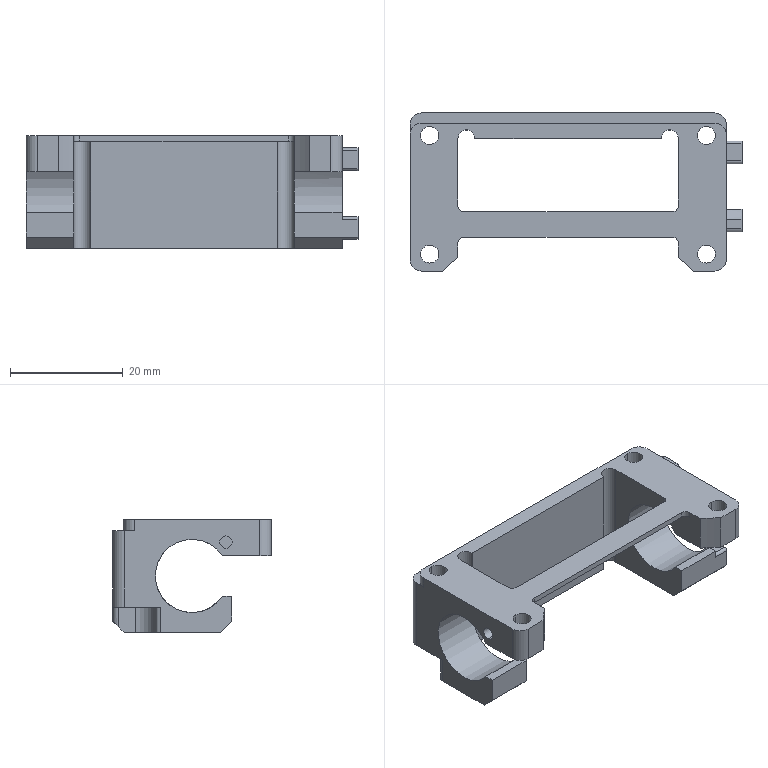NC program | Mastercam | posted with a generic post | part box 58.8 x 28 x 20 mm
Lines 58 to 1155 of 29451:
(10 FEM |TOOL - 10|DIA. OFF. - 10|LEN. - 10|TOOL DIA. - 10.)
N182 T10 M6
N184 G0 G54 G90 X44.9 Y11.6 C0. B0. S6500 M3
N186 G43 H10 Z25.
N188 Z5.
N190 G1 Z0. F600.
N192 X34.9 F4000.
N194 X28.421
N196 X27.5
N198 G3 X27.503 Y11.8 I-6.677 J.2
N200 X27.331 Y13.306 I-6.68
N202 X22.397 Y17.14 I-4.94 J-1.266
N204 G1 X-19.603
N206 G3 X-24.686 Y12.372 I.004 J-5.098
N208 X-24.702 Y11.824 I9.387 J-.548
N210 X-24.7 Y11.6 I9.403
N212 X-25.137 Y11.607 I-.437 J-14.093
N214 X-26.331 Y11.556 J-14.1
N216 X-31.497 Y7.059 I.769 J-6.099
N218 X-31.7 Y5.553 I6.076 J-1.583
N220 G1 Y-4.947
N222 Y-4.999
N224 G3 X-26.909 Y-10.131 I5.144
N226 G1 X-26.591 Y-10.14
N228 X-18.113
N230 G3 X-13.146 Y-6.056 I-.016 J5.083
N232 X-13.035 Y-4.999 I-4.996 J1.057
N234 G1 Y-4.967
N236 Y4.401
N238 X15.835
N240 Y-4.947
N242 Y-4.999
N244 G3 X20.626 Y-10.131 I5.144
N246 G1 X20.944 Y-10.14
N248 X29.422
N250 G3 X34.389 Y-6.056 I-.016 J5.083
N252 X34.5 Y-4.999 I-4.993 J1.057
N254 G1 Y-4.976
N256 Y5.5
N258 G3 X30.664 Y11.164 I-6.149 J-.033
N260 X28.421 Y11.6 I-2.297 J-5.835
N262 G2 X30.664 Y11.164 I-.054 J-6.271
N264 X34.5 Y5.5 I-2.313 J-5.697
N266 G1 Y-4.976
N268 Y-4.999
N270 G2 X34.389 Y-6.056 I-5.104
N272 X29.422 Y-10.14 I-4.983 J.999
N274 G1 X20.944
N276 X20.626 Y-10.131
N278 G2 X15.835 Y-4.999 I.353 J5.132
N280 G1 Y-4.947
N282 Y2.121
N284 X1.735 Y-8.5
N286 X.501 Y-9.
N288 X2.308
N290 X9.335 Y-2.
N292 X-6.535
N294 X-6.035 Y-3.5
N296 Y-5.
N298 X-6.048 Y-5.5
N300 X-6.087 Y-6.
N302 X-6.203 Y-7.
N304 X-6.296 Y-7.5
N306 X-6.414 Y-8.
N308 X-6.56 Y-8.5
N310 X-6.895 Y-9.5
N312 X-7.104 Y-10.
N314 X-7.347 Y-10.5
N316 X-7.628 Y-11.
N318 X-8.242 Y-12.
N320 X-9.644 Y-13.
N322 X-13.997 Y-14.5
N324 X-28.109 Y-15.
N326 X27.9
N328 X16.824 Y-14.5
N330 X12.468 Y-13.
N332 X11.058 Y-12.
N334 X10.733 Y-11.5
N336 X10.158 Y-10.5
N338 X9.913 Y-10.
N340 X9.702 Y-9.5
N342 X9.523 Y-9.
N344 X9.215 Y-8.
N346 X9.095 Y-7.5
N348 X9.003 Y-7.
N350 X8.938 Y-6.5
N352 X8.848 Y-5.5
N354 X8.835 Y-5.
N356 Y-4.
N358 X9.335 Y-2.
N360 X16.101 Y-6.631
N362 G3 X20.626 Y-10.131 I4.878 J1.632
N364 G1 X20.944 Y-10.14
N366 X21.227
N368 X34.9 Y-19.5
N370 Y19.5
N372 X-34.9
N374 Y-19.5
N376 X34.9
N378 G0 Z5.
N380 Z25.
N382 X44.9 Y11.6
N384 Z4.414
N386 G1 Z-.586 F600.
N388 X34.9 F4000.
N390 X28.426
N392 X27.5
N394 G3 X27.509 Y12.093 I-12.959 J.493
N396 X27.46 Y13.223 I-12.968
N398 X23.346 Y17.637 I-5.119 J-.647
N400 X22.4 Y17.726 I-.946 J-4.973
N402 G1 X22.397
N404 X-19.603
N406 G3 X-24.686 Y12.957 I.004 J-5.098
N408 X-24.708 Y12.119 I16.278 J-.838
N410 X-24.7 Y11.6 I16.3
N412 X-25.137 Y11.607 I-.437 J-13.987
N414 X-26.336 Y11.555 J-13.994
N416 X-31.57 Y6.748 I.77 J-6.091
N418 X-31.7 Y5.553 I7.039 J-1.369
N420 G1 Y-5.533
N422 Y-5.585
N424 G3 X-26.909 Y-10.717 I5.144
N426 G1 X-26.591 Y-10.726
N428 X-18.126
N430 G3 X-13.053 Y-6.01 I-.01 J5.098
N432 X-13.035 Y-5.586 I-5.082 J.424
N434 G1 Y4.401
N436 X15.835
N438 Y-5.533
N440 Y-5.585
N442 G3 X20.626 Y-10.717 I5.144
N444 G1 X20.944 Y-10.726
N446 X29.409
N448 G3 X34.482 Y-6.01 I-.01 J5.098
N450 X34.5 Y-5.586 I-5.082 J.424
N452 G1 Y5.504
N454 G3 X30.364 Y11.274 I-6.14 J-.034
N456 X28.426 Y11.6 I-2.012 J-6.031
N458 G1 X27.5
N460 X28.426
N462 G2 X30.364 Y11.274 I-.074 J-6.357
N464 X34.5 Y5.504 I-2.004 J-5.804
N466 G1 Y-5.586
N468 G2 X34.482 Y-6.01 I-5.1
N470 X29.409 Y-10.726 I-5.083 J.382
N472 G1 X20.944
N474 X20.626 Y-10.717
N476 G2 X15.835 Y-5.585 I.353 J5.132
N478 G1 Y-5.533
N480 Y4.401
N482 X12.048
N484 X-13.372 Y-7.443
N486 G2 X-18.126 Y-10.726 I-4.764 J1.815
N488 G1 X-20.418
N490 X-29.591 Y-15.
N492 X1.663 Y-8.5
N494 X.805
N496 X2.001
N498 X9.335 Y-2.
N500 X-6.535
N502 X-6.035 Y-3.5
N504 Y-5.5
N506 X-6.044 Y-6.
N508 X-6.078 Y-6.5
N510 X-6.187 Y-7.5
N512 X-6.273 Y-8.
N514 X-6.387 Y-8.5
N516 X-6.529 Y-9.
N518 X-6.859 Y-10.
N520 X-7.063 Y-10.5
N522 X-7.301 Y-11.
N524 X-7.575 Y-11.5
N526 X-8.986 Y-13.
N528 X-13.615 Y-14.5
N530 X16.441
N532 X11.807 Y-13.
N534 X10.682 Y-12.
N536 X10.114 Y-11.
N538 X9.874 Y-10.5
N540 X9.669 Y-10.
N542 X9.495 Y-9.5
N544 X9.193 Y-8.5
N546 X9.078 Y-8.
N548 X8.99 Y-7.5
N550 X8.929 Y-7.
N552 X8.844 Y-6.
N554 X8.835 Y-5.5
N556 Y-3.5
N558 X9.335 Y-2.
N560 X15.918 Y-6.506
N562 G3 X20.626 Y-10.717 I5.061 J.921
N564 G1 X20.944 Y-10.726
N566 X22.083
N568 X34.9 Y-19.5
N570 Y19.5
N572 X-34.9
N574 Y-19.5
N576 X34.9
N578 G0 Z4.414
N580 Z25.
N582 X27.236 Y29.5
N584 Z3.829
N586 G1 Z-1.171 F600.
N588 Y19.5 F4000.
N590 Y14.741
N592 G3 X25.868 Y16.918 I-5.03 J-1.642
N594 X22.365 Y18.311 I-3.508 J-3.723
N596 G1 X3.073 Y18.312
N598 X1.823 Y18.313
N600 X-4.083 Y18.312
N602 G3 X-5.36 Y18.313 I-1.277 J-732.939
N604 X-6.588 Y18.312 J-732.94
N606 X-7.288 Y18.313 I-.7 J-235.219
N608 X-8.017 Y18.312 J-235.22
N610 X-8.697 Y18.313 I-.68 J-317.868
N612 X-9.377 Y18.312 J-317.869
N614 G1 X-19.388
N616 X-19.408
N618 X-19.438
N620 X-19.457 Y18.313
N622 X-19.476 Y18.312
N624 X-19.499 Y18.313
N626 G3 X-21.136 Y18.062 I.07 J-5.92
N628 X-24.686 Y13.372 I1.604 J-4.903
N630 G1 X-24.7 Y13.053
N632 Y11.6
N634 G3 X-25.137 Y11.607 I-.437 J-14.066
N636 X-26.331 Y11.556 J-14.073
N638 X-31.497 Y7.059 I.769 J-6.099
N640 X-31.7 Y5.553 I6.075 J-1.583
N642 G1 Y-6.119
N644 Y-6.17
N646 G3 X-26.909 Y-11.302 I5.144
N648 G1 X-26.591 Y-11.312
N650 X-18.126
N652 G3 X-13.053 Y-6.596 I-.01 J5.098
N654 X-13.035 Y-6.171 I-5.082 J.425
N656 G1 Y4.401
N658 X15.835
N660 Y-6.119
N662 Y-6.17
N664 G3 X20.626 Y-11.302 I5.144
N666 G1 X20.944 Y-11.312
N668 X29.409
N670 G3 X34.482 Y-6.596 I-.01 J5.098
N672 X34.5 Y-6.171 I-5.082 J.425
N674 G1 Y5.509
N676 G3 X29.934 Y11.404 I-6.137 J-.037
N678 X28.426 Y11.6 I-1.564 J-6.137
N680 G1 X27.5
N682 G3 X27.509 Y12.3 I-27.475 J.7
N684 X27.49 Y13.319 I-27.484
N686 X27.236 Y14.741 I-5.705 J-.284
N688 G2 X27.49 Y13.319 I-5.451 J-1.706
N690 X27.509 Y12.3 I-27.465 J-1.019
N692 X27.5 Y11.6 I-27.484
N694 G1 X28.426
N696 G2 X29.934 Y11.404 I-.056 J-6.333
N698 X34.5 Y5.509 I-1.571 J-5.932
N700 G1 Y-6.171
N702 G2 X34.482 Y-6.596 I-5.1
N704 X29.409 Y-11.312 I-5.083 J.382
N706 G1 X20.944
N708 X20.626 Y-11.302
N710 G2 X15.835 Y-6.17 I.353 J5.132
N712 G1 Y-6.119
N714 Y4.4
N716 X1.614 Y-8.5
N718 X.934
N720 X1.87
N722 X9.335 Y-2.
N724 X-6.535
N726 X-6.035 Y-3.5
N728 Y-6.
N730 X-6.041 Y-6.5
N732 X-6.071 Y-7.
N734 X-6.175 Y-8.
N736 X-6.257 Y-8.5
N738 X-6.365 Y-9.
N740 X-6.502 Y-9.5
N742 X-6.827 Y-10.5
N744 X-7.025 Y-11.
N746 X-7.257 Y-11.5
N748 X-8.029 Y-12.5
N750 X-11.823 Y-14.5
N752 X14.65
N754 X10.847 Y-12.5
N756 X10.07 Y-11.5
N758 X9.837 Y-11.
N760 X9.637 Y-10.5
N762 X9.468 Y-10.
N764 X9.171 Y-9.
N766 X9.061 Y-8.5
N768 X8.978 Y-8.
N770 X8.921 Y-7.5
N772 X8.841 Y-6.5
N774 X8.835 Y-6.
N776 Y-3.5
N778 X9.335 Y-2.
N780 X15.843 Y-6.455
N782 G3 X20.626 Y-11.302 I5.136 J.285
N784 G1 X20.944 Y-11.312
N786 X22.938
N788 X34.9 Y-19.5
N790 Y19.5
N792 X-34.9
N794 Y-19.5
N796 X34.9
N798 G0 Z3.829
N800 Z25.
N802 X25.369 Y29.5
N804 Z3.243
N806 G1 Z-1.757 F600.
N808 Y19.5 F4000.
N810 Y17.627
N812 G3 X21.945 Y18.898 I-3.424 J-3.975
N814 G1 X21.94
N816 G3 X20.816 Y18.9 I-1.124 J-452.637
N818 X19.19 Y18.898 J-452.638
N820 X17.39 Y18.903 I-1.8 J-322.689
N822 X15.589 Y18.898 J-322.694
N824 G1 X-18.884
N826 G3 X-19.084 Y18.902 I-.2 J-5.411
N828 X-22.47 Y17.712 J-5.415
N830 X-24.7 Y13.053 I3.808 J-4.686
N832 G1 Y11.6
N834 G3 X-25.138 Y11.607 I-.438 J-14.051
N836 X-26.331 Y11.556 J-14.058
N838 X-31.497 Y7.059 I.769 J-6.099
N840 X-31.7 Y5.553 I6.075 J-1.583
N842 G1 Y1.439
N844 G3 X-33.303 Y.168 I2.049 J-4.231
N846 X-34.5 Y-3.094 I3.939 J-3.295
N848 G1 Y-6.704
N850 Y-6.756
N852 G3 X-29.709 Y-11.888 I5.144
N854 G1 X-29.391 Y-11.898
N856 X-18.126
N858 G3 X-13.053 Y-7.181 I-.01 J5.098
N860 X-13.035 Y-6.757 I-5.082 J.424
N862 G1 Y4.401
N864 X15.835
N866 Y-6.704
N868 Y-6.756
N870 G3 X20.626 Y-11.888 I5.144
N872 G1 X20.944 Y-11.898
N874 X29.409
N876 G3 X34.482 Y-7.181 I-.01 J5.098
N878 X34.5 Y-6.757 I-5.082 J.424
N880 G1 Y5.513
N882 G3 X29.184 Y11.549 I-6.13 J-.039
N884 X28.426 Y11.6 I-.829 J-6.718
N886 G1 X27.5
N888 G3 X27.509 Y12.299 I-27.561 J.699
N890 X27.49 Y13.319 I-27.57
N892 X25.369 Y17.627 I-6.057 J-.305
N894 G2 X27.49 Y13.319 I-3.936 J-4.613
N896 X27.509 Y12.299 I-27.551 J-1.02
N898 X27.5 Y11.6 I-27.57
N900 G1 X28.426
N902 G2 X29.184 Y11.549 I-.071 J-6.769
N904 X34.5 Y5.513 I-.814 J-6.075
N906 G1 Y-6.757
N908 G2 X34.482 Y-7.181 I-5.1
N910 X29.409 Y-11.898 I-5.083 J.381
N912 G1 X20.944
N914 X20.626 Y-11.888
N916 G2 X15.835 Y-6.756 I.353 J5.132
N918 G1 Y-6.704
N920 Y4.401
N922 X13.005
N924 X1.412 Y-8.
N926 X1.392
N928 X1.249 Y-8.5
N930 X1.542
N932 X1.412 Y-8.
N934 X9.335 Y-2.
N936 X-6.535
N938 X-6.035 Y-3.5
N940 Y-6.5
N942 X-6.038 Y-7.
N944 X-6.064 Y-7.5
N946 X-6.114 Y-8.
N948 X-6.241 Y-9.
N950 X-6.344 Y-9.5
N952 X-6.477 Y-10.
N954 X-6.796 Y-11.
N956 X-6.989 Y-11.5
N958 X-7.215 Y-12.
N960 X-7.477 Y-12.5
N962 X-10.857 Y-14.
N964 X13.683
N966 X10.582 Y-13.
N968 X10.028 Y-12.
N970 X9.8 Y-11.5
N972 X9.606 Y-11.
N974 X9.442 Y-10.5
N976 X9.15 Y-9.5
N978 X9.044 Y-9.
N980 X8.966 Y-8.5
N982 X8.914 Y-8.
N984 X8.838 Y-7.
N986 X8.835 Y-6.5
N988 Y-3.5
N990 X9.335 Y-2.
N992 X15.835 Y-6.449
N994 Y-6.704
N996 Y-6.756
N998 G3 X20.626 Y-11.888 I5.144
N1000 G1 X20.944 Y-11.898
N1002 X23.794
N1004 X34.9 Y-19.5
N1006 Y19.5
N1008 X-34.9
N1010 Y-19.5
N1012 X34.9
N1014 G0 Z3.243
N1016 Z25.
N1018 X23.661 Y29.5
N1020 Z2.657
N1022 G1 Z-2.343 F600.
N1024 Y19.5 F4000.
N1026 Y18.665
N1028 G3 X21.426 Y19.1 I-2.298 J-5.855
N1030 G1 X-18.576
N1032 G3 X-24.647 Y13.801 I.002 J-6.129
N1034 X-24.7 Y13.053 I6.469 J-.833
N1036 G1 Y11.6
N1038 G3 X-25.138 Y11.607 I-.438 J-14.035
N1040 X-26.331 Y11.556 J-14.042
N1042 X-31.497 Y7.059 I.769 J-6.099
N1044 X-31.7 Y5.553 I6.075 J-1.583
N1046 G1 Y1.549
N1048 G3 X-33.304 Y.281 I2.051 J-4.243
N1050 X-34.5 Y-2.956 I3.901 J-3.28
N1052 G1 Y-6.947
N1054 Y-6.999
N1056 G3 X-29.479 Y-12.099 I5.101
N1058 G1 X-18.212
N1060 G3 X-18.134 Y-12.1 I.078 J5.098
N1062 X-13.035 Y-7.001 J5.099
N1064 G1 Y-7.
N1066 Y4.401
N1068 X15.835
N1070 Y-6.947
N1072 Y-6.999
N1074 G3 X20.856 Y-12.099 I5.101
N1076 G1 X29.323
N1078 G3 X29.401 Y-12.1 I.078 J5.098
N1080 X34.5 Y-7.001 J5.099
N1082 G1 Y-7.
N1084 Y5.5
N1086 G3 X30.664 Y11.164 I-6.148 J-.033
N1088 X28.426 Y11.6 I-2.297 J-5.835
N1090 G1 X27.5
N1092 G3 X27.509 Y12.299 I-27.648 J.699
N1094 X27.49 Y13.319 I-27.657
N1096 X23.661 Y18.665 I-6.075 J-.306
N1098 G2 X27.49 Y13.319 I-2.246 J-5.652
N1100 X27.509 Y12.299 I-27.638 J-1.02
N1102 X27.5 Y11.6 I-27.657
N1104 G1 X28.426
N1106 G2 X30.664 Y11.164 I-.059 J-6.271
N1108 X34.5 Y5.5 I-2.312 J-5.697
N1110 G1 Y-7.
N1112 Y-7.001
N1114 G2 X29.401 Y-12.1 I-5.099
N1116 X29.323 Y-12.099 J5.099
N1118 G1 X20.856
N1120 G2 X15.835 Y-6.999 I.08 J5.1
N1122 G1 X15.836 Y-6.947
N1124 X15.835 Y4.401
N1126 X11.751
N1128 X1.397 Y-8.
N1130 X1.28 Y-8.5
N1132 X1.513
N1134 X1.397 Y-8.
N1136 X9.335 Y-2.
N1138 X-6.535
N1140 X-6.035 Y-3.5
N1142 Y-7.
N1144 X-6.048 Y-7.5
N1146 X-6.087 Y-8.
N1148 X-6.203 Y-9.
N1150 X-6.296 Y-9.5
N1152 X-6.416 Y-10.
N1154 X-6.566 Y-10.5
N1156 X-6.904 Y-11.5
N1158 X-7.116 Y-12.
N1160 X-7.363 Y-12.5
N1162 X-10.536 Y-14.
N1164 X13.338
N1166 X10.164 Y-12.5
N1168 X9.917 Y-12.
N1170 X9.705 Y-11.5
N1172 X9.525 Y-11.
N1174 X9.217 Y-10.
N1176 X9.096 Y-9.5
N1178 X9.004 Y-9.
N1180 X8.938 Y-8.5
N1182 X8.848 Y-7.5
N1184 X8.835 Y-7.
N1186 Y-3.5
N1188 X9.335 Y-2.
N1190 X15.835 Y-6.449
N1192 Y-6.947
N1194 Y-6.999
N1196 G3 X20.856 Y-12.099 I5.101
N1198 G1 X24.089
N1200 X34.9 Y-19.5
N1202 Y19.5
N1204 X-34.9
N1206 Y-19.5
N1208 X34.9
N1210 G0 Z2.657
N1212 Z25.
N1214 X23.957 Y29.5
N1216 Z2.071
N1218 G1 Z-2.929 F600.
N1220 Y19.5 F4000.
N1222 Y18.536
N1224 G3 X21.426 Y19.1 I-2.562 J-5.537
N1226 G1 X-18.581
N1228 G3 X-24.7 Y13.053 I.004 J-6.124
N1230 G1 Y11.6
N1232 G3 X-25.137 Y11.607 I-.437 J-14.093
N1234 X-26.331 Y11.556 J-14.1
N1236 X-31.497 Y7.059 I.769 J-6.099
N1238 X-31.7 Y5.553 I6.075 J-1.583
N1240 G1 Y1.549
N1242 G3 X-33.307 Y.278 I2.07 J-4.268
N1244 X-34.5 Y-2.956 I3.898 J-3.275
N1246 G1 Y-6.947
N1248 X-34.469 Y-7.56
N1250 X-34.365 Y-8.165
N1252 X-34.189 Y-8.753
N1254 X-33.943 Y-9.316
N1256 X-33.632 Y-9.845
N1258 X-33.26 Y-10.333
N1260 X-32.831 Y-10.772
N1262 X-32.353 Y-11.157
N1264 X-31.832 Y-11.482
N1266 X-31.276 Y-11.742
N1268 X-30.693 Y-11.934
N1270 X-30.091 Y-12.054
N1272 X-29.479 Y-12.099
N1274 X-18.207
N1276 G3 X-18.131 Y-12.1 I.076 J5.096
N1278 X-13.034 Y-7.003 J5.097
N1280 G1 Y-7.
N1282 X-13.035 Y4.401
N1284 X15.835
N1286 Y-6.947
N1288 X15.866 Y-7.56
N1290 X15.97 Y-8.165
N1292 X16.146 Y-8.753
N1294 X16.392 Y-9.316
N1296 X16.703 Y-9.845
N1298 X17.075 Y-10.333
N1300 X17.504 Y-10.772
N1302 X17.982 Y-11.157
N1304 X18.503 Y-11.482
N1306 X19.059 Y-11.742
N1308 X19.642 Y-11.934
N1310 X20.244 Y-12.054
N1312 X20.856 Y-12.099
N1314 X29.328
N1316 G3 X29.404 Y-12.1 I.076 J5.096
N1318 X34.501 Y-7.003 J5.097
N1320 G1 Y-7.
N1322 X34.5 Y5.5
N1324 G3 X30.664 Y11.164 I-6.148 J-.033
N1326 X28.426 Y11.6 I-2.297 J-5.835
N1328 G1 X27.5
N1330 G3 X27.509 Y12.298 I-27.734 J.698
N1332 X27.49 Y13.319 I-27.743
N1334 X23.957 Y18.536 I-6.071 J-.306
N1336 G2 X27.49 Y13.319 I-2.538 J-5.523
N1338 X27.509 Y12.298 I-27.724 J-1.021
N1340 X27.5 Y11.6 I-27.743
N1342 G1 X28.426
N1344 G2 X30.664 Y11.164 I-.059 J-6.271
N1346 X34.5 Y5.5 I-2.312 J-5.697
N1348 G1 Y-7.
N1350 Y-7.003
N1352 G2 X29.404 Y-12.099 I-5.096
N1354 G1 X29.328 Y-12.098
N1356 X20.856 Y-12.099
N1358 X20.244 Y-12.052
N1360 X19.642 Y-11.932
N1362 X19.059 Y-11.741
N1364 X18.503 Y-11.481
N1366 X17.983 Y-11.156
N1368 X17.505 Y-10.771
N1370 X17.077 Y-10.332
N1372 X16.704 Y-9.844
N1374 X16.393 Y-9.315
N1376 X16.148 Y-8.752
N1378 X15.972 Y-8.165
N1380 X15.867 Y-7.56
N1382 X15.835 Y-6.947
N1384 Y4.401
N1386 X11.939
N1388 X1.397 Y-8.
N1390 X1.28 Y-8.5
N1392 X1.514
N1394 X1.397 Y-8.
N1396 X9.335 Y-2.
N1398 X-6.535
N1400 X-6.035 Y-3.5
N1402 Y-7.
N1404 X-6.048 Y-7.5
N1406 X-6.087 Y-8.
N1408 X-6.203 Y-9.
N1410 X-6.296 Y-9.5
N1412 X-6.416 Y-10.
N1414 X-6.565 Y-10.5
N1416 X-6.903 Y-11.5
N1418 X-7.116 Y-12.
N1420 X-7.362 Y-12.5
N1422 X-10.535 Y-14.
N1424 X13.339
N1426 X10.165 Y-12.5
N1428 X9.918 Y-12.
N1430 X9.706 Y-11.5
N1432 X9.525 Y-11.
N1434 X9.218 Y-10.
N1436 X9.097 Y-9.5
N1438 X9.004 Y-9.
N1440 X8.938 Y-8.5
N1442 X8.848 Y-7.5
N1444 X8.835 Y-7.
N1446 Y-3.5
N1448 X9.335 Y-2.
N1450 X15.835 Y-6.449
N1452 Y-6.947
N1454 X15.866 Y-7.56
N1456 X15.97 Y-8.165
N1458 X16.146 Y-8.753
N1460 X16.392 Y-9.316
N1462 X16.703 Y-9.845
N1464 X17.075 Y-10.333
N1466 X17.504 Y-10.772
N1468 X17.982 Y-11.157
N1470 X18.503 Y-11.482
N1472 X19.059 Y-11.742
N1474 X19.642 Y-11.934
N1476 X20.244 Y-12.054
N1478 X20.856 Y-12.099
N1480 X24.089
N1482 X34.9 Y-19.5
N1484 Y19.5
N1486 X-34.9
N1488 Y-19.5
N1490 X34.9
N1492 G0 Z2.071
N1494 Z25.
N1496 X23.957 Y29.5
N1498 Z1.486
N1500 G1 Z-3.514 F600.
N1502 Y19.5 F4000.
N1504 Y18.536
N1506 G3 X21.426 Y19.1 I-2.562 J-5.537
N1508 G1 X-18.585
N1510 G3 X-24.7 Y13.053 I.006 J-6.122
N1512 G1 Y11.6
N1514 G3 X-25.137 Y11.607 I-.437 J-14.093
N1516 X-26.331 Y11.556 J-14.1
N1518 X-31.497 Y7.059 I.769 J-6.099
N1520 X-31.7 Y5.553 I6.075 J-1.583
N1522 G1 Y1.549
N1524 G3 X-33.09 Y.52 I2.011 J-4.171
N1526 X-34.5 Y-2.956 I3.69 J-3.52
N1528 G1 Y-6.947
N1530 Y-7.
N1532 G3 X-29.479 Y-12.099 I5.1
N1534 G1 X-18.203
N1536 G3 X-18.129 Y-12.1 I.074 J5.093
N1538 X-13.035 Y-7.006 J5.094
N1540 G1 Y-7.
N1542 Y4.401
N1544 X15.835
N1546 Y-6.947
N1548 Y-7.
N1550 G3 X20.856 Y-12.099 I5.1
N1552 G1 X29.332
N1554 G3 X29.406 Y-12.1 I.074 J5.093
N1556 X34.5 Y-7.006 J5.094
N1558 G1 Y-7.
N1560 Y5.5
N1562 G3 X30.664 Y11.164 I-6.148 J-.033
N1564 X28.426 Y11.6 I-2.297 J-5.835
N1566 G1 X27.5
N1568 G3 X27.509 Y12.3 I-27.45 J.7
N1570 X27.49 Y13.319 I-27.459
N1572 X23.957 Y18.536 I-6.071 J-.306
N1574 G2 X27.49 Y13.319 I-2.538 J-5.523
N1576 X27.509 Y12.3 I-27.44 J-1.019
N1578 X27.5 Y11.6 I-27.459
N1580 G1 X28.426
N1582 G2 X30.664 Y11.164 I-.059 J-6.271
N1584 X34.5 Y5.5 I-2.312 J-5.697
N1586 G1 Y-7.
N1588 Y-7.006
N1590 G2 X29.406 Y-12.1 I-5.094
N1592 X29.332 Y-12.099 J5.094
N1594 G1 X20.856
N1596 G2 X15.835 Y-7. I.079 J5.099
N1598 G1 X15.836 Y-6.947
N1600 X15.835 Y4.401
N1602 X11.939
N1604 X1.397 Y-8.
N1606 X1.28 Y-8.5
N1608 X1.513
N1610 X1.397 Y-8.
N1612 X9.335 Y-2.
N1614 X-6.535
N1616 X-6.035 Y-3.5
N1618 Y-7.
N1620 X-6.048 Y-7.5
N1622 X-6.087 Y-8.
N1624 X-6.203 Y-9.
N1626 X-6.295 Y-9.5
N1628 X-6.415 Y-10.
N1630 X-6.565 Y-10.5
N1632 X-6.903 Y-11.5
N1634 X-7.115 Y-12.
N1636 X-7.362 Y-12.5
N1638 X-10.533 Y-14.
N1640 X13.337
N1642 X10.164 Y-12.5
N1644 X9.917 Y-12.
N1646 X9.704 Y-11.5
N1648 X9.525 Y-11.
N1650 X9.217 Y-10.
N1652 X9.096 Y-9.5
N1654 X9.003 Y-9.
N1656 X8.938 Y-8.5
N1658 X8.848 Y-7.5
N1660 X8.835 Y-7.
N1662 Y-3.5
N1664 X9.335 Y-2.
N1666 X15.835 Y-6.449
N1668 Y-6.947
N1670 Y-7.
N1672 G3 X20.856 Y-12.099 I5.1
N1674 G1 X24.089
N1676 X34.9 Y-19.5
N1678 Y19.5
N1680 X-34.9
N1682 Y-19.5
N1684 X34.9
N1686 G0 Z1.486
N1688 Z25.
N1690 X23.664 Y29.5
N1692 Z.9
N1694 G1 Z-4.1 F600.
N1696 Y19.5 F4000.
N1698 Y18.664
N1700 G3 X21.426 Y19.1 I-2.302 J-5.86
N1702 G1 X-18.589
N1704 G3 X-24.7 Y13.053 I.008 J-6.119
N1706 G1 Y11.6
N1708 G3 X-25.137 Y11.607 I-.437 J-14.093
N1710 X-26.331 Y11.556 J-14.1
N1712 X-31.497 Y7.059 I.769 J-6.099
N1714 X-31.7 Y5.553 I6.075 J-1.583
N1716 G1 Y1.549
N1718 G3 X-33.09 Y.52 I2.011 J-4.171
N1720 X-34.5 Y-2.956 I3.69 J-3.52
N1722 G1 Y-6.947
N1724 Y-7.
N1726 G3 X-29.479 Y-12.099 I5.1
N1728 G1 X-18.198
N1730 X-18.127
N1732 G3 X-13.036 Y-7.008 J5.091
N1734 G1 Y-7.
N1736 X-13.035 Y4.401
N1738 X15.835
N1740 Y-6.947
N1742 Y-7.
N1744 G3 X20.856 Y-12.099 I5.1
N1746 G1 X29.337
N1748 X29.408
N1750 G3 X34.499 Y-7.008 J5.091
N1752 G1 Y-7.
N1754 X34.5 Y5.5
N1756 G3 X30.664 Y11.164 I-6.148 J-.033
N1758 X28.426 Y11.6 I-2.297 J-5.835
N1760 G1 X27.5
N1762 G3 X27.509 Y12.3 I-27.45 J.7
N1764 X27.49 Y13.319 I-27.459
N1766 X23.664 Y18.664 I-6.075 J-.306
N1768 G2 X27.49 Y13.319 I-2.249 J-5.651
N1770 X27.509 Y12.3 I-27.44 J-1.019
N1772 X27.5 Y11.6 I-27.459
N1774 G1 X28.426
N1776 G2 X30.664 Y11.164 I-.059 J-6.271
N1778 X34.5 Y5.5 I-2.312 J-5.697
N1780 G1 Y-7.
N1782 Y-7.008
N1784 G2 X29.408 Y-12.1 I-5.092
N1786 X29.337 Y-12.099 J5.092
N1788 G1 X20.856
N1790 G2 X15.835 Y-7. I.079 J5.099
N1792 G1 X15.836 Y-6.947
N1794 X15.835 Y4.401
N1796 X11.753
N1798 X1.397 Y-8.
N1800 X1.281 Y-8.5
N1802 X1.513
N1804 X1.397 Y-8.
N1806 X9.335 Y-2.
N1808 X-6.535
N1810 X-6.035 Y-3.5
N1812 Y-7.
N1814 X-6.048 Y-7.5
N1816 X-6.086 Y-8.
N1818 X-6.202 Y-9.
N1820 X-6.295 Y-9.5
N1822 X-6.415 Y-10.
N1824 X-6.564 Y-10.5
N1826 X-6.902 Y-11.5
N1828 X-7.114 Y-12.
N1830 X-7.361 Y-12.5
N1832 X-10.532 Y-14.
N1834 X13.337
N1836 X10.164 Y-12.5
N1838 X9.917 Y-12.
N1840 X9.704 Y-11.5
N1842 X9.525 Y-11.
N1844 X9.217 Y-10.
N1846 X9.096 Y-9.5
N1848 X9.003 Y-9.
N1850 X8.938 Y-8.5
N1852 X8.848 Y-7.5
N1854 X8.835 Y-7.
N1856 Y-3.5
N1858 X9.335 Y-2.
N1860 X15.835 Y-6.449
N1862 Y-6.947
N1864 Y-7.
N1866 G3 X20.856 Y-12.099 I5.1
N1868 G1 X24.089
N1870 X34.9 Y-19.5
N1872 Y19.5
N1874 X-34.9
N1876 Y-19.5
N1878 X34.9
N1880 G0 Z.9
N1882 Z25.
N1884 X44.9 Y16.25
N1886 Z.314
N1888 G1 Z-4.686 F600.
N1890 X34.9 F4000.
N1892 X33.085
N1894 G3 X30.354 Y18.454 I-5.731 J-4.306
N1896 X28.454 Y19.019 I-2.856 J-6.135
N1898 G1 X28.44 Y19.02
N1900 G3 X27.518 Y19.101 I-.922 J-5.223
N1902 X27.426 Y19.1 J-5.304
N1904 G1 X-24.575
N1906 G3 X-25.677 Y19.014 I.042 J-7.68
N1908 X-26.574 Y19.1 I-.903 J-4.714
N1910 G1 X-29.375
N1912 X-29.401
N1914 G3 X-34.5 Y14.053 J-5.099
N1916 G1 Y-6.947
N1918 Y-7.
N1920 G3 X-29.479 Y-12.099 I5.1
N1922 G1 X-18.194
N1924 X-18.125
N1926 G3 X-13.036 Y-7.01 J5.089
N1928 G1 Y-7.
N1930 X-13.035 Y4.401
N1932 X15.835
N1934 Y-6.947
N1936 Y-7.
N1938 G3 X20.856 Y-12.099 I5.1
N1940 G1 X29.341
N1942 X29.41
N1944 G3 X34.499 Y-7.01 J5.089
N1946 G1 Y-7.
N1948 X34.5 Y12.001
N1950 G3 X34.303 Y13.654 I-7.722 J-.082
N1952 G1 X34.3 Y13.664
N1954 G3 X33.991 Y14.638 I-5.208 J-1.114
N1956 X33.085 Y16.25 I-6.757 J-2.74
N1958 G2 X33.991 Y14.638 I-5.851 J-4.352
N1960 X34.3 Y13.664 I-4.899 J-2.088
N1962 G1 X34.303 Y13.654
N1964 G2 X34.5 Y12.001 I-7.525 J-1.735
N1966 G1 Y-7.
N1968 Y-7.01
N1970 G2 X29.41 Y-12.1 I-5.09
N1972 X29.341 Y-12.099 J5.09
N1974 G1 X20.856
N1976 G2 X15.835 Y-7. I.079 J5.099
N1978 G1 X15.836 Y-6.947
N1980 X15.835 Y3.049
N1982 X1.397 Y-8.
N1984 X1.281 Y-8.5
N1986 X1.513
N1988 X1.397 Y-8.
N1990 X9.335 Y-2.
N1992 X-6.535
N1994 X-6.035 Y-3.5
N1996 Y-7.
N1998 X-6.048 Y-7.5
N2000 X-6.086 Y-8.
N2002 X-6.202 Y-9.
N2004 X-6.294 Y-9.5
N2006 X-6.414 Y-10.
N2008 X-6.564 Y-10.5
N2010 X-6.901 Y-11.5
N2012 X-7.113 Y-12.
N2014 X-7.36 Y-12.5
N2016 X-10.531 Y-14.
N2018 X13.337
N2020 X10.164 Y-12.5
N2022 X9.917 Y-12.
N2024 X9.704 Y-11.5
N2026 X9.525 Y-11.
N2028 X9.217 Y-10.
N2030 X9.096 Y-9.5
N2032 X9.003 Y-9.
N2034 X8.938 Y-8.5
N2036 X8.848 Y-7.5
N2038 X8.835 Y-7.
N2040 Y-3.5
N2042 X9.335 Y-2.
N2044 X15.835 Y-6.449
N2046 Y-6.947
N2048 Y-7.
N2050 G3 X20.856 Y-12.099 I5.1
N2052 G1 X24.089
N2054 X34.9 Y-19.5
N2056 Y19.5
N2058 X-34.9
N2060 Y-19.5
N2062 X34.9
N2064 G0 Z.314
N2066 Z25.
N2068 X44.9 Y16.25
N2070 Z-.271
N2072 G1 Z-5.271 F600.
N2074 X34.9 F4000.
N2076 X33.085
N2078 G3 X30.354 Y18.454 I-5.731 J-4.306
N2080 X28.454 Y19.019 I-2.864 J-6.163
N2082 G1 X28.44 Y19.02
N2084 G3 X27.518 Y19.101 I-.922 J-5.223
N2086 X27.426 Y19.1 J-5.304
N2088 G1 X-24.579
N2090 G3 X-25.677 Y19.014 I.043 J-7.649
N2092 X-26.574 Y19.1 I-.903 J-4.714
N2094 G1 X-29.379
N2096 X-29.403
N2098 G3 X-34.5 Y14.053 J-5.097
N2100 G1 Y-6.947
N2102 Y-7.
N2104 G3 X-29.479 Y-12.099 I5.1
N2106 G1 X-18.19
N2108 X-18.122
N2110 G3 X-13.035 Y-7.012 J5.087
N2112 G1 Y-7.
N2114 Y4.401
N2116 X15.835
N2118 Y-6.947
N2120 Y-7.
N2122 G3 X20.856 Y-12.099 I5.1
N2124 G1 X29.345
N2126 X29.413
N2128 G3 X34.5 Y-7.012 J5.087
N2130 G1 Y-7.
N2132 Y12.006
N2134 G3 X34.303 Y13.654 I-7.702 J-.085
N2136 G1 X34.3 Y13.664
N2138 G3 X33.99 Y14.642 I-5.207 J-1.114
N2140 X33.085 Y16.25 I-6.741 J-2.735
N2142 G2 X33.99 Y14.642 I-5.836 J-4.343
N2144 X34.3 Y13.664 I-4.897 J-2.092
N2146 G1 X34.303 Y13.654
N2148 G2 X34.5 Y12.006 I-7.505 J-1.733
N2150 G1 Y-7.
N2152 Y-7.012
N2154 G2 X29.413 Y-12.099 I-5.087
N2156 G1 X29.345
N2158 X20.856
N2160 G2 X15.835 Y-7. I.079 J5.099
N2162 G1 X15.836 Y-6.947
N2164 X15.835 Y3.049
N2166 X1.397 Y-8.
N2168 X1.281 Y-8.5
N2170 X1.513
N2172 X1.397 Y-8.
N2174 X9.335 Y-2.
N2176 X-6.535
N2178 X-6.035 Y-3.5
N2180 Y-7.
N2182 X-6.047 Y-7.5
N2184 X-6.086 Y-8.
N2186 X-6.202 Y-9.
N2188 X-6.294 Y-9.5
N2190 X-6.414 Y-10.
N2192 X-6.563 Y-10.5
N2194 X-6.901 Y-11.5
N2196 X-7.113 Y-12.
N2198 X-7.359 Y-12.5
N2200 X-10.529 Y-14.
N2202 X13.337
N2204 X10.164 Y-12.5
N2206 X9.917 Y-12.
N2208 X9.704 Y-11.5
N2210 X9.525 Y-11.
N2212 X9.217 Y-10.
N2214 X9.096 Y-9.5
N2216 X9.003 Y-9.
N2218 X8.938 Y-8.5
N2220 X8.848 Y-7.5
N2222 X8.835 Y-7.
N2224 Y-3.5
N2226 X9.335 Y-2.
N2228 X15.835 Y-6.449
N2230 Y-6.947
N2232 Y-7.
N2234 G3 X20.856 Y-12.099 I5.1
N2236 G1 X24.089
N2238 X34.9 Y-19.5
N2240 Y19.5
N2242 X-34.9
N2244 Y-19.5
N2246 X34.9
N2248 G0 Z-.271
N2250 Z25.
N2252 X44.9 Y16.25
N2254 Z-.857
N2256 G1 Z-5.857 F600.
N2258 X34.9 F4000.
N2260 X33.085
N2262 G3 X30.354 Y18.454 I-5.731 J-4.306
N2264 X28.454 Y19.019 I-2.853 J-6.126
N2266 G1 X28.44 Y19.02
N2268 G3 X27.518 Y19.101 I-.922 J-5.223
N2270 X27.426 Y19.1 J-5.304
N2272 G1 X-24.584
N2274 G3 X-25.677 Y19.014 I.045 J-7.619
N2276 X-26.574 Y19.1 I-.903 J-4.714
N2278 G1 X-29.384
N2280 X-29.405
N2282 G3 X-34.5 Y14.053 J-5.095
N2284 G1 Y-6.947
N2286 Y-7.
N2288 G3 X-29.479 Y-12.099 I5.1
N2290 G1 X-18.185
N2292 X-18.12
N2294 G3 X-13.035 Y-7.014 J5.085
N2296 G1 Y-7.
N2298 Y4.401
N2300 X15.835
N2302 Y-6.947
N2304 Y-7.
N2306 G3 X20.856 Y-12.099 I5.1
N2308 G1 X29.35
N2310 X29.415
N2312 G3 X34.5 Y-7.014 J5.085
N2314 G1 Y-7.
N2316 Y12.01
N2318 G3 X34.303 Y13.654 I-7.681 J-.086
N2320 G1 X34.3 Y13.664
N2322 G3 X33.988 Y14.646 I-5.206 J-1.114
N2324 X33.085 Y16.25 I-6.724 J-2.73
N2326 G2 X33.988 Y14.646 I-5.821 J-4.334
N2328 X34.3 Y13.664 I-4.894 J-2.096
N2330 G1 X34.303 Y13.654
N2332 G2 X34.5 Y12.01 I-7.484 J-1.73
N2334 G1 Y-7.
N2336 Y-7.014
N2338 G2 X29.415 Y-12.099 I-5.085
N2340 G1 X29.35
N2342 X20.856
N2344 G2 X15.835 Y-7. I.079 J5.099
N2346 G1 X15.836 Y-6.947
N2348 X15.835 Y3.049
N2350 X1.397 Y-8.
N2352 X1.281 Y-8.5
N2354 X1.513
N2356 X1.397 Y-8.
N2358 X9.335 Y-2.
N2360 X-6.535
N2362 X-6.035 Y-3.5
N2364 Y-7.
N2366 X-6.047 Y-7.5
N2368 X-6.086 Y-8.
N2370 X-6.201 Y-9.
N2372 X-6.293 Y-9.5
N2374 X-6.413 Y-10.